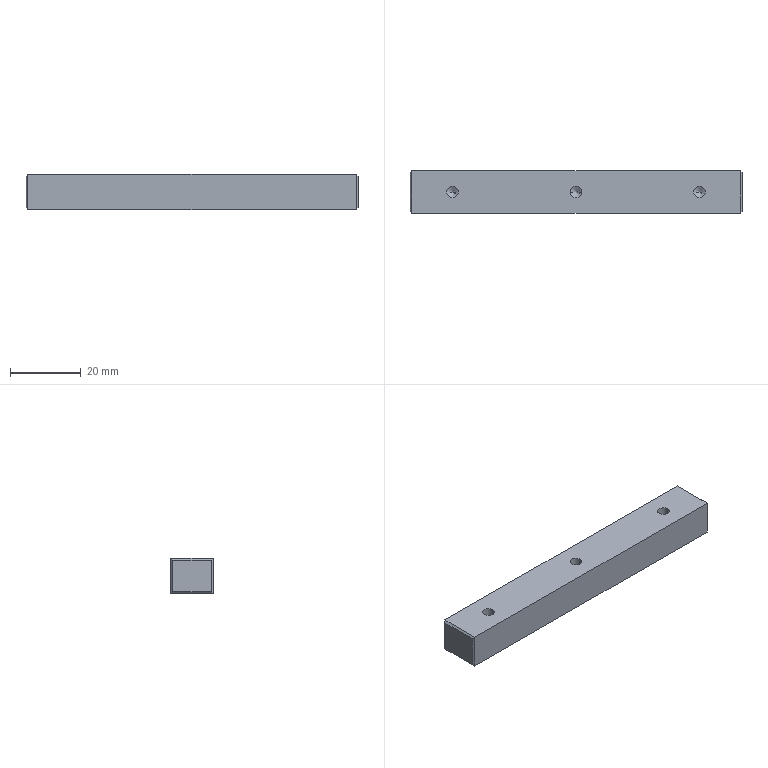Part | STEP file | GLSJ-10-40 | 1 solid | 26 faces | box 94 x 12 x 10 mm | volume 11056 mm3 | plane 14 | cylinder 6 | cone 6 | commonest cylinder face diameters 3.3 x6